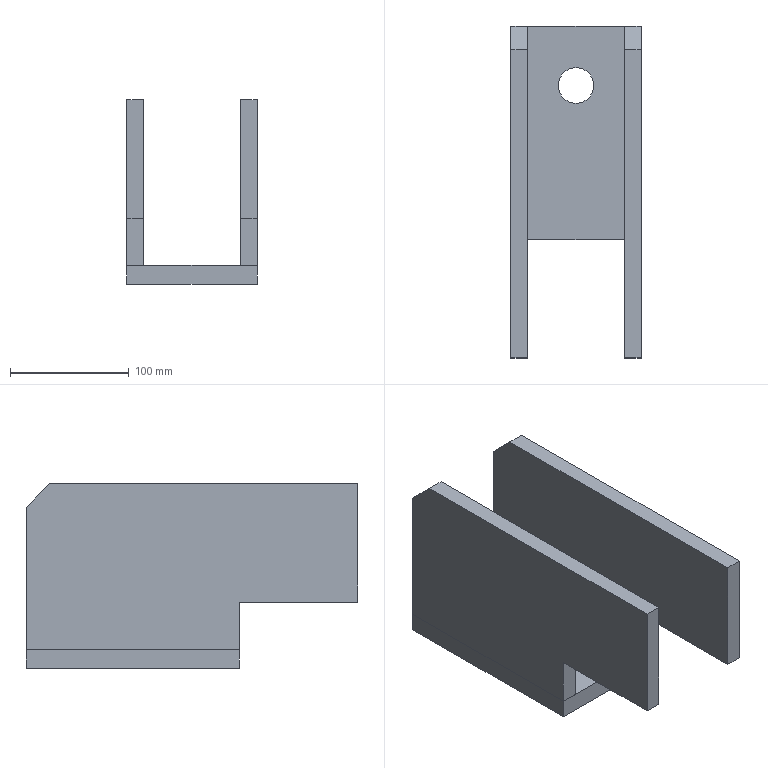Part | SolidWorks | features ICE 3, Chamfer 1, Extrusion 1, MirrorSolid 1, WeldmentFeature 1 | 3 solids | 26 faces | box 110 x 280 x 156 mm | volume 1285490 mm3 | plane 24 | cylinder 2 | commonest cylinder face diameters 30 x2
STEP:
#1=CARTESIAN_POINT('',(-55.,50.,136.));
#2=VERTEX_POINT('',#1);
#3=CARTESIAN_POINT('',(-55.,50.,16.));
#4=VERTEX_POINT('',#3);
#5=CARTESIAN_POINT('',(-55.,50.,16.));
#6=DIRECTION('',(0.,0.,-1.));
#7=VECTOR('',#6,1000.);
#8=LINE('',#5,#7);
#9=EDGE_CURVE('',#2,#4,#8,.T.);
#10=ORIENTED_EDGE('',*,*,#9,.F.);
#11=CARTESIAN_POINT('',(-41.,50.,136.));
#12=VERTEX_POINT('',#11);
#13=CARTESIAN_POINT('',(-41.,50.,136.));
#14=DIRECTION('',(1.,0.,0.));
#15=VECTOR('',#14,1000.);
#16=LINE('',#13,#15);
#17=EDGE_CURVE('',#2,#12,#16,.T.);
#18=ORIENTED_EDGE('',*,*,#17,.T.);
#19=CARTESIAN_POINT('',(-41.,50.,16.));
#20=VERTEX_POINT('',#19);
#21=CARTESIAN_POINT('',(-41.,50.,16.));
#22=DIRECTION('',(0.,0.,-1.));
#23=VECTOR('',#22,1000.);
#24=LINE('',#21,#23);
#25=EDGE_CURVE('',#12,#20,#24,.T.);
#26=ORIENTED_EDGE('',*,*,#25,.T.);
#27=CARTESIAN_POINT('',(-41.,50.,16.));
#28=DIRECTION('',(-1.,0.,0.));
#29=VECTOR('',#28,1000.);
#30=LINE('',#27,#29);
#31=EDGE_CURVE('',#20,#4,#30,.T.);
#32=ORIENTED_EDGE('',*,*,#31,.T.);
#33=EDGE_LOOP('',(#10,#18,#26,#32));
#34=FACE_OUTER_BOUND('',#33,.T.);
#35=CARTESIAN_POINT('',(-41.,50.,16.));
#36=DIRECTION('',(0.,1.,0.));
#37=DIRECTION('',(0.,0.,1.));
#38=AXIS2_PLACEMENT_3D('',#35,#36,#37);
#39=PLANE('',#38);
#40=ADVANCED_FACE('',(#34),#39,.T.);
#41=CARTESIAN_POINT('',(-41.,-230.,156.));
#42=VERTEX_POINT('',#41);
#43=CARTESIAN_POINT('',(-41.,30.,156.));
#44=VERTEX_POINT('',#43);
#45=CARTESIAN_POINT('',(-41.,50.,156.));
#46=DIRECTION('',(0.,1.,0.));
#47=VECTOR('',#46,1000.);
#48=LINE('',#45,#47);
#49=EDGE_CURVE('',#42,#44,#48,.T.);
#50=ORIENTED_EDGE('',*,*,#49,.T.);
#51=CARTESIAN_POINT('',(-55.,30.,156.));
#52=VERTEX_POINT('',#51);
#53=CARTESIAN_POINT('',(-41.,30.,156.));
#54=DIRECTION('',(-1.,0.,0.));
#55=VECTOR('',#54,1000.);
#56=LINE('',#53,#55);
#57=EDGE_CURVE('',#44,#52,#56,.T.);
#58=ORIENTED_EDGE('',*,*,#57,.T.);
#59=CARTESIAN_POINT('',(-55.,-230.,156.));
#60=VERTEX_POINT('',#59);
#61=CARTESIAN_POINT('',(-55.,50.,156.));
#62=DIRECTION('',(0.,1.,0.));
#63=VECTOR('',#62,1000.);
#64=LINE('',#61,#63);
#65=EDGE_CURVE('',#60,#52,#64,.T.);
#66=ORIENTED_EDGE('',*,*,#65,.F.);
#67=CARTESIAN_POINT('',(-41.,-230.,156.));
#68=DIRECTION('',(-1.,0.,0.));
#69=VECTOR('',#68,1000.);
#70=LINE('',#67,#69);
#71=EDGE_CURVE('',#42,#60,#70,.T.);
#72=ORIENTED_EDGE('',*,*,#71,.F.);
#73=EDGE_LOOP('',(#50,#58,#66,#72));
#74=FACE_OUTER_BOUND('',#73,.T.);
#75=CARTESIAN_POINT('',(-41.,50.,156.));
#76=DIRECTION('',(0.,0.,1.));
#77=DIRECTION('',(0.,-1.,0.));
#78=AXIS2_PLACEMENT_3D('',#75,#76,#77);
#79=PLANE('',#78);
#80=ADVANCED_FACE('',(#74),#79,.T.);
#81=CARTESIAN_POINT('',(-55.,-230.,56.));
#82=VERTEX_POINT('',#81);
#83=CARTESIAN_POINT('',(-55.,-230.,156.));
#84=DIRECTION('',(0.,0.,1.));
#85=VECTOR('',#84,1000.);
#86=LINE('',#83,#85);
#87=EDGE_CURVE('',#82,#60,#86,.T.);
#88=ORIENTED_EDGE('',*,*,#87,.F.);
#89=CARTESIAN_POINT('',(-41.,-230.,56.));
#90=VERTEX_POINT('',#89);
#91=CARTESIAN_POINT('',(-41.,-230.,56.));
#92=DIRECTION('',(-1.,0.,0.));
#93=VECTOR('',#92,1000.);
#94=LINE('',#91,#93);
#95=EDGE_CURVE('',#90,#82,#94,.T.);
#96=ORIENTED_EDGE('',*,*,#95,.F.);
#97=CARTESIAN_POINT('',(-41.,-230.,156.));
#98=DIRECTION('',(0.,0.,1.));
#99=VECTOR('',#98,1000.);
#100=LINE('',#97,#99);
#101=EDGE_CURVE('',#90,#42,#100,.T.);
#102=ORIENTED_EDGE('',*,*,#101,.T.);
#103=ORIENTED_EDGE('',*,*,#71,.T.);
#104=EDGE_LOOP('',(#88,#96,#102,#103));
#105=FACE_OUTER_BOUND('',#104,.T.);
#106=CARTESIAN_POINT('',(-41.,-230.,156.));
#107=DIRECTION('',(0.,-1.,0.));
#108=DIRECTION('',(0.,0.,-1.));
#109=AXIS2_PLACEMENT_3D('',#106,#107,#108);
#110=PLANE('',#109);
#111=ADVANCED_FACE('',(#105),#110,.T.);
#112=CARTESIAN_POINT('',(-55.,-130.,56.));
#113=VERTEX_POINT('',#112);
#114=CARTESIAN_POINT('',(-55.,-230.,56.));
#115=DIRECTION('',(0.,-1.,0.));
#116=VECTOR('',#115,1000.);
#117=LINE('',#114,#116);
#118=EDGE_CURVE('',#113,#82,#117,.T.);
#119=ORIENTED_EDGE('',*,*,#118,.F.);
#120=CARTESIAN_POINT('',(-41.,-130.,56.));
#121=VERTEX_POINT('',#120);
#122=CARTESIAN_POINT('',(-41.,-130.,56.));
#123=DIRECTION('',(-1.,0.,0.));
#124=VECTOR('',#123,1000.);
#125=LINE('',#122,#124);
#126=EDGE_CURVE('',#121,#113,#125,.T.);
#127=ORIENTED_EDGE('',*,*,#126,.F.);
#128=CARTESIAN_POINT('',(-41.,-230.,56.));
#129=DIRECTION('',(0.,-1.,0.));
#130=VECTOR('',#129,1000.);
#131=LINE('',#128,#130);
#132=EDGE_CURVE('',#121,#90,#131,.T.);
#133=ORIENTED_EDGE('',*,*,#132,.T.);
#134=ORIENTED_EDGE('',*,*,#95,.T.);
#135=EDGE_LOOP('',(#119,#127,#133,#134));
#136=FACE_OUTER_BOUND('',#135,.T.);
#137=CARTESIAN_POINT('',(-41.,-230.,56.));
#138=DIRECTION('',(0.,0.,-1.));
#139=DIRECTION('',(-1.,0.,0.));
#140=AXIS2_PLACEMENT_3D('',#137,#138,#139);
#141=PLANE('',#140);
#142=ADVANCED_FACE('',(#136),#141,.T.);
#143=CARTESIAN_POINT('',(-55.,-130.,16.));
#144=VERTEX_POINT('',#143);
#145=CARTESIAN_POINT('',(-55.,-130.,56.));
#146=DIRECTION('',(0.,0.,1.));
#147=VECTOR('',#146,1000.);
#148=LINE('',#145,#147);
#149=EDGE_CURVE('',#144,#113,#148,.T.);
#150=ORIENTED_EDGE('',*,*,#149,.F.);
#151=CARTESIAN_POINT('',(-41.,-130.,16.));
#152=VERTEX_POINT('',#151);
#153=CARTESIAN_POINT('',(-41.,-130.,16.));
#154=DIRECTION('',(-1.,0.,0.));
#155=VECTOR('',#154,1000.);
#156=LINE('',#153,#155);
#157=EDGE_CURVE('',#152,#144,#156,.T.);
#158=ORIENTED_EDGE('',*,*,#157,.F.);
#159=CARTESIAN_POINT('',(-41.,-130.,56.));
#160=DIRECTION('',(0.,0.,1.));
#161=VECTOR('',#160,1000.);
#162=LINE('',#159,#161);
#163=EDGE_CURVE('',#152,#121,#162,.T.);
#164=ORIENTED_EDGE('',*,*,#163,.T.);
#165=ORIENTED_EDGE('',*,*,#126,.T.);
#166=EDGE_LOOP('',(#150,#158,#164,#165));
#167=FACE_OUTER_BOUND('',#166,.T.);
#168=CARTESIAN_POINT('',(-41.,-130.,56.));
#169=DIRECTION('',(0.,-1.,0.));
#170=DIRECTION('',(0.,0.,-1.));
#171=AXIS2_PLACEMENT_3D('',#168,#169,#170);
#172=PLANE('',#171);
#173=ADVANCED_FACE('',(#167),#172,.T.);
#174=CARTESIAN_POINT('',(-55.,50.,16.));
#175=DIRECTION('',(0.,-1.,0.));
#176=VECTOR('',#175,1000.);
#177=LINE('',#174,#176);
#178=EDGE_CURVE('',#4,#144,#177,.T.);
#179=ORIENTED_EDGE('',*,*,#178,.F.);
#180=ORIENTED_EDGE('',*,*,#31,.F.);
#181=CARTESIAN_POINT('',(-41.,50.,16.));
#182=DIRECTION('',(0.,-1.,0.));
#183=VECTOR('',#182,1000.);
#184=LINE('',#181,#183);
#185=EDGE_CURVE('',#20,#152,#184,.T.);
#186=ORIENTED_EDGE('',*,*,#185,.T.);
#187=ORIENTED_EDGE('',*,*,#157,.T.);
#188=EDGE_LOOP('',(#179,#180,#186,#187));
#189=FACE_OUTER_BOUND('',#188,.T.);
#190=CARTESIAN_POINT('',(-41.,50.,16.));
#191=DIRECTION('',(0.,0.,-1.));
#192=DIRECTION('',(-1.,0.,0.));
#193=AXIS2_PLACEMENT_3D('',#190,#191,#192);
#194=PLANE('',#193);
#195=ADVANCED_FACE('',(#189),#194,.T.);
#196=ORIENTED_EDGE('',*,*,#25,.F.);
#197=CARTESIAN_POINT('',(-41.,93.,93.));
#198=DIRECTION('',(0.,-0.7071,0.7071));
#199=VECTOR('',#198,1000.);
#200=LINE('',#197,#199);
#201=EDGE_CURVE('',#12,#44,#200,.T.);
#202=ORIENTED_EDGE('',*,*,#201,.T.);
#203=ORIENTED_EDGE('',*,*,#49,.F.);
#204=ORIENTED_EDGE('',*,*,#101,.F.);
#205=ORIENTED_EDGE('',*,*,#132,.F.);
#206=ORIENTED_EDGE('',*,*,#163,.F.);
#207=ORIENTED_EDGE('',*,*,#185,.F.);
#208=EDGE_LOOP('',(#196,#202,#203,#204,#205,#206,#207));
#209=FACE_OUTER_BOUND('',#208,.T.);
#210=CARTESIAN_POINT('',(-41.,0.,0.));
#211=DIRECTION('',(1.,0.,0.));
#212=DIRECTION('',(0.,0.,-1.));
#213=AXIS2_PLACEMENT_3D('',#210,#211,#212);
#214=PLANE('',#213);
#215=ADVANCED_FACE('',(#209),#214,.T.);
#216=ORIENTED_EDGE('',*,*,#65,.T.);
#217=CARTESIAN_POINT('',(-55.,30.,156.));
#218=DIRECTION('',(0.,0.7071,-0.7071));
#219=VECTOR('',#218,1000.);
#220=LINE('',#217,#219);
#221=EDGE_CURVE('',#52,#2,#220,.T.);
#222=ORIENTED_EDGE('',*,*,#221,.T.);
#223=ORIENTED_EDGE('',*,*,#9,.T.);
#224=ORIENTED_EDGE('',*,*,#178,.T.);
#225=ORIENTED_EDGE('',*,*,#149,.T.);
#226=ORIENTED_EDGE('',*,*,#118,.T.);
#227=ORIENTED_EDGE('',*,*,#87,.T.);
#228=EDGE_LOOP('',(#216,#222,#223,#224,#225,#226,#227));
#229=FACE_OUTER_BOUND('',#228,.T.);
#230=CARTESIAN_POINT('',(-55.,0.,0.));
#231=DIRECTION('',(1.,0.,0.));
#232=DIRECTION('',(0.,0.,-1.));
#233=AXIS2_PLACEMENT_3D('',#230,#231,#232);
#234=PLANE('',#233);
#235=ADVANCED_FACE('',(#229),#234,.F.);
#236=ORIENTED_EDGE('',*,*,#201,.F.);
#237=ORIENTED_EDGE('',*,*,#17,.F.);
#238=ORIENTED_EDGE('',*,*,#221,.F.);
#239=ORIENTED_EDGE('',*,*,#57,.F.);
#240=EDGE_LOOP('',(#236,#237,#238,#239));
#241=FACE_OUTER_BOUND('',#240,.T.);
#242=CARTESIAN_POINT('',(-41.,30.,156.));
#243=DIRECTION('',(0.,-0.7071,-0.7071));
#244=DIRECTION('',(-1.,0.,0.));
#245=AXIS2_PLACEMENT_3D('',#242,#243,#244);
#246=PLANE('',#245);
#247=ADVANCED_FACE('',(#241),#246,.F.);
#248=CLOSED_SHELL('',(#40,#80,#111,#142,#173,#195,#215,#235,#247));
#249=MANIFOLD_SOLID_BREP('',#248);
#250=CARTESIAN_POINT('',(55.,50.,136.));
#251=VERTEX_POINT('',#250);
#252=CARTESIAN_POINT('',(55.,50.,16.));
#253=VERTEX_POINT('',#252);
#254=CARTESIAN_POINT('',(55.,50.,16.));
#255=DIRECTION('',(0.,0.,-1.));
#256=VECTOR('',#255,1000.);
#257=LINE('',#254,#256);
#258=EDGE_CURVE('',#251,#253,#257,.T.);
#259=ORIENTED_EDGE('',*,*,#258,.T.);
#260=CARTESIAN_POINT('',(41.,50.,16.));
#261=VERTEX_POINT('',#260);
#262=CARTESIAN_POINT('',(41.,50.,16.));
#263=DIRECTION('',(1.,0.,0.));
#264=VECTOR('',#263,1000.);
#265=LINE('',#262,#264);
#266=EDGE_CURVE('',#261,#253,#265,.T.);
#267=ORIENTED_EDGE('',*,*,#266,.F.);
#268=CARTESIAN_POINT('',(41.,50.,136.));
#269=VERTEX_POINT('',#268);
#270=CARTESIAN_POINT('',(41.,50.,16.));
#271=DIRECTION('',(0.,0.,-1.));
#272=VECTOR('',#271,1000.);
#273=LINE('',#270,#272);
#274=EDGE_CURVE('',#269,#261,#273,.T.);
#275=ORIENTED_EDGE('',*,*,#274,.F.);
#276=CARTESIAN_POINT('',(41.,50.,136.));
#277=DIRECTION('',(-1.,0.,0.));
#278=VECTOR('',#277,1000.);
#279=LINE('',#276,#278);
#280=EDGE_CURVE('',#251,#269,#279,.T.);
#281=ORIENTED_EDGE('',*,*,#280,.F.);
#282=EDGE_LOOP('',(#259,#267,#275,#281));
#283=FACE_OUTER_BOUND('',#282,.T.);
#284=CARTESIAN_POINT('',(41.,50.,16.));
#285=DIRECTION('',(0.,1.,0.));
#286=DIRECTION('',(0.,0.,1.));
#287=AXIS2_PLACEMENT_3D('',#284,#285,#286);
#288=PLANE('',#287);
#289=ADVANCED_FACE('',(#283),#288,.T.);
#290=CARTESIAN_POINT('',(41.,-230.,156.));
#291=VERTEX_POINT('',#290);
#292=CARTESIAN_POINT('',(41.,30.,156.));
#293=VERTEX_POINT('',#292);
#294=CARTESIAN_POINT('',(41.,50.,156.));
#295=DIRECTION('',(0.,1.,0.));
#296=VECTOR('',#295,1000.);
#297=LINE('',#294,#296);
#298=EDGE_CURVE('',#291,#293,#297,.T.);
#299=ORIENTED_EDGE('',*,*,#298,.F.);
#300=CARTESIAN_POINT('',(55.,-230.,156.));
#301=VERTEX_POINT('',#300);
#302=CARTESIAN_POINT('',(41.,-230.,156.));
#303=DIRECTION('',(1.,0.,0.));
#304=VECTOR('',#303,1000.);
#305=LINE('',#302,#304);
#306=EDGE_CURVE('',#291,#301,#305,.T.);
#307=ORIENTED_EDGE('',*,*,#306,.T.);
#308=CARTESIAN_POINT('',(55.,30.,156.));
#309=VERTEX_POINT('',#308);
#310=CARTESIAN_POINT('',(55.,50.,156.));
#311=DIRECTION('',(0.,1.,0.));
#312=VECTOR('',#311,1000.);
#313=LINE('',#310,#312);
#314=EDGE_CURVE('',#301,#309,#313,.T.);
#315=ORIENTED_EDGE('',*,*,#314,.T.);
#316=CARTESIAN_POINT('',(41.,30.,156.));
#317=DIRECTION('',(1.,0.,0.));
#318=VECTOR('',#317,1000.);
#319=LINE('',#316,#318);
#320=EDGE_CURVE('',#293,#309,#319,.T.);
#321=ORIENTED_EDGE('',*,*,#320,.F.);
#322=EDGE_LOOP('',(#299,#307,#315,#321));
#323=FACE_OUTER_BOUND('',#322,.T.);
#324=CARTESIAN_POINT('',(41.,50.,156.));
#325=DIRECTION('',(0.,0.,1.));
#326=DIRECTION('',(0.,-1.,0.));
#327=AXIS2_PLACEMENT_3D('',#324,#325,#326);
#328=PLANE('',#327);
#329=ADVANCED_FACE('',(#323),#328,.T.);
#330=CARTESIAN_POINT('',(55.,-230.,56.));
#331=VERTEX_POINT('',#330);
#332=CARTESIAN_POINT('',(55.,-230.,156.));
#333=DIRECTION('',(0.,0.,1.));
#334=VECTOR('',#333,1000.);
#335=LINE('',#332,#334);
#336=EDGE_CURVE('',#331,#301,#335,.T.);
#337=ORIENTED_EDGE('',*,*,#336,.T.);
#338=ORIENTED_EDGE('',*,*,#306,.F.);
#339=CARTESIAN_POINT('',(41.,-230.,56.));
#340=VERTEX_POINT('',#339);
#341=CARTESIAN_POINT('',(41.,-230.,156.));
#342=DIRECTION('',(0.,0.,1.));
#343=VECTOR('',#342,1000.);
#344=LINE('',#341,#343);
#345=EDGE_CURVE('',#340,#291,#344,.T.);
#346=ORIENTED_EDGE('',*,*,#345,.F.);
#347=CARTESIAN_POINT('',(41.,-230.,56.));
#348=DIRECTION('',(1.,0.,0.));
#349=VECTOR('',#348,1000.);
#350=LINE('',#347,#349);
#351=EDGE_CURVE('',#340,#331,#350,.T.);
#352=ORIENTED_EDGE('',*,*,#351,.T.);
#353=EDGE_LOOP('',(#337,#338,#346,#352));
#354=FACE_OUTER_BOUND('',#353,.T.);
#355=CARTESIAN_POINT('',(41.,-230.,156.));
#356=DIRECTION('',(0.,-1.,0.));
#357=DIRECTION('',(0.,0.,-1.));
#358=AXIS2_PLACEMENT_3D('',#355,#356,#357);
#359=PLANE('',#358);
#360=ADVANCED_FACE('',(#354),#359,.T.);
#361=CARTESIAN_POINT('',(55.,-130.,56.));
#362=VERTEX_POINT('',#361);
#363=CARTESIAN_POINT('',(55.,-230.,56.));
#364=DIRECTION('',(0.,-1.,0.));
#365=VECTOR('',#364,1000.);
#366=LINE('',#363,#365);
#367=EDGE_CURVE('',#362,#331,#366,.T.);
#368=ORIENTED_EDGE('',*,*,#367,.T.);
#369=ORIENTED_EDGE('',*,*,#351,.F.);
#370=CARTESIAN_POINT('',(41.,-130.,56.));
#371=VERTEX_POINT('',#370);
#372=CARTESIAN_POINT('',(41.,-230.,56.));
#373=DIRECTION('',(0.,-1.,0.));
#374=VECTOR('',#373,1000.);
#375=LINE('',#372,#374);
#376=EDGE_CURVE('',#371,#340,#375,.T.);
#377=ORIENTED_EDGE('',*,*,#376,.F.);
#378=CARTESIAN_POINT('',(41.,-130.,56.));
#379=DIRECTION('',(1.,0.,0.));
#380=VECTOR('',#379,1000.);
#381=LINE('',#378,#380);
#382=EDGE_CURVE('',#371,#362,#381,.T.);
#383=ORIENTED_EDGE('',*,*,#382,.T.);
#384=EDGE_LOOP('',(#368,#369,#377,#383));
#385=FACE_OUTER_BOUND('',#384,.T.);
#386=CARTESIAN_POINT('',(41.,-230.,56.));
#387=DIRECTION('',(0.,0.,-1.));
#388=DIRECTION('',(1.,0.,0.));
#389=AXIS2_PLACEMENT_3D('',#386,#387,#388);
#390=PLANE('',#389);
#391=ADVANCED_FACE('',(#385),#390,.T.);
#392=CARTESIAN_POINT('',(55.,-130.,16.));
#393=VERTEX_POINT('',#392);
#394=CARTESIAN_POINT('',(55.,-130.,56.));
#395=DIRECTION('',(0.,0.,1.));
#396=VECTOR('',#395,1000.);
#397=LINE('',#394,#396);
#398=EDGE_CURVE('',#393,#362,#397,.T.);
#399=ORIENTED_EDGE('',*,*,#398,.T.);
#400=ORIENTED_EDGE('',*,*,#382,.F.);
#401=CARTESIAN_POINT('',(41.,-130.,16.));
#402=VERTEX_POINT('',#401);
#403=CARTESIAN_POINT('',(41.,-130.,56.));
#404=DIRECTION('',(0.,0.,1.));
#405=VECTOR('',#404,1000.);
#406=LINE('',#403,#405);
#407=EDGE_CURVE('',#402,#371,#406,.T.);
#408=ORIENTED_EDGE('',*,*,#407,.F.);
#409=CARTESIAN_POINT('',(41.,-130.,16.));
#410=DIRECTION('',(1.,0.,0.));
#411=VECTOR('',#410,1000.);
#412=LINE('',#409,#411);
#413=EDGE_CURVE('',#402,#393,#412,.T.);
#414=ORIENTED_EDGE('',*,*,#413,.T.);
#415=EDGE_LOOP('',(#399,#400,#408,#414));
#416=FACE_OUTER_BOUND('',#415,.T.);
#417=CARTESIAN_POINT('',(41.,-130.,56.));
#418=DIRECTION('',(0.,-1.,0.));
#419=DIRECTION('',(0.,0.,-1.));
#420=AXIS2_PLACEMENT_3D('',#417,#418,#419);
#421=PLANE('',#420);
#422=ADVANCED_FACE('',(#416),#421,.T.);
#423=CARTESIAN_POINT('',(55.,50.,16.));
#424=DIRECTION('',(0.,-1.,0.));
#425=VECTOR('',#424,1000.);
#426=LINE('',#423,#425);
#427=EDGE_CURVE('',#253,#393,#426,.T.);
#428=ORIENTED_EDGE('',*,*,#427,.T.);
#429=ORIENTED_EDGE('',*,*,#413,.F.);
#430=CARTESIAN_POINT('',(41.,50.,16.));
#431=DIRECTION('',(0.,-1.,0.));
#432=VECTOR('',#431,1000.);
#433=LINE('',#430,#432);
#434=EDGE_CURVE('',#261,#402,#433,.T.);
#435=ORIENTED_EDGE('',*,*,#434,.F.);
#436=ORIENTED_EDGE('',*,*,#266,.T.);
#437=EDGE_LOOP('',(#428,#429,#435,#436));
#438=FACE_OUTER_BOUND('',#437,.T.);
#439=CARTESIAN_POINT('',(41.,50.,16.));
#440=DIRECTION('',(0.,0.,-1.));
#441=DIRECTION('',(1.,0.,0.));
#442=AXIS2_PLACEMENT_3D('',#439,#440,#441);
#443=PLANE('',#442);
#444=ADVANCED_FACE('',(#438),#443,.T.);
#445=ORIENTED_EDGE('',*,*,#274,.T.);
#446=ORIENTED_EDGE('',*,*,#434,.T.);
#447=ORIENTED_EDGE('',*,*,#407,.T.);
#448=ORIENTED_EDGE('',*,*,#376,.T.);
#449=ORIENTED_EDGE('',*,*,#345,.T.);
#450=ORIENTED_EDGE('',*,*,#298,.T.);
#451=CARTESIAN_POINT('',(41.,93.,93.));
#452=DIRECTION('',(0.,-0.7071,0.7071));
#453=VECTOR('',#452,1000.);
#454=LINE('',#451,#453);
#455=EDGE_CURVE('',#269,#293,#454,.T.);
#456=ORIENTED_EDGE('',*,*,#455,.F.);
#457=EDGE_LOOP('',(#445,#446,#447,#448,#449,#450,#456));
#458=FACE_OUTER_BOUND('',#457,.T.);
#459=CARTESIAN_POINT('',(41.,0.,0.));
#460=DIRECTION('',(-1.,0.,0.));
#461=DIRECTION('',(0.,0.,-1.));
#462=AXIS2_PLACEMENT_3D('',#459,#460,#461);
#463=PLANE('',#462);
#464=ADVANCED_FACE('',(#458),#463,.T.);
#465=ORIENTED_EDGE('',*,*,#314,.F.);
#466=ORIENTED_EDGE('',*,*,#336,.F.);
#467=ORIENTED_EDGE('',*,*,#367,.F.);
#468=ORIENTED_EDGE('',*,*,#398,.F.);
#469=ORIENTED_EDGE('',*,*,#427,.F.);
#470=ORIENTED_EDGE('',*,*,#258,.F.);
#471=CARTESIAN_POINT('',(55.,30.,156.));
#472=DIRECTION('',(0.,0.7071,-0.7071));
#473=VECTOR('',#472,1000.);
#474=LINE('',#471,#473);
#475=EDGE_CURVE('',#309,#251,#474,.T.);
#476=ORIENTED_EDGE('',*,*,#475,.F.);
#477=EDGE_LOOP('',(#465,#466,#467,#468,#469,#470,#476));
#478=FACE_OUTER_BOUND('',#477,.T.);
#479=CARTESIAN_POINT('',(55.,0.,0.));
#480=DIRECTION('',(-1.,0.,0.));
#481=DIRECTION('',(0.,0.,-1.));
#482=AXIS2_PLACEMENT_3D('',#479,#480,#481);
#483=PLANE('',#482);
#484=ADVANCED_FACE('',(#478),#483,.F.);
#485=ORIENTED_EDGE('',*,*,#455,.T.);
#486=ORIENTED_EDGE('',*,*,#320,.T.);
#487=ORIENTED_EDGE('',*,*,#475,.T.);
#488=ORIENTED_EDGE('',*,*,#280,.T.);
#489=EDGE_LOOP('',(#485,#486,#487,#488));
#490=FACE_OUTER_BOUND('',#489,.T.);
#491=CARTESIAN_POINT('',(41.,30.,156.));
#492=DIRECTION('',(0.,-0.7071,-0.7071));
#493=DIRECTION('',(1.,0.,0.));
#494=AXIS2_PLACEMENT_3D('',#491,#492,#493);
#495=PLANE('',#494);
#496=ADVANCED_FACE('',(#490),#495,.F.);
#497=CLOSED_SHELL('',(#289,#329,#360,#391,#422,#444,#464,#484,#496));
#498=MANIFOLD_SOLID_BREP('',#497);
#499=CARTESIAN_POINT('',(-15.,0.,16.));
#500=VERTEX_POINT('',#499);
#501=CARTESIAN_POINT('',(15.,0.,16.));
#502=VERTEX_POINT('',#501);
#503=CARTESIAN_POINT('',(0.,0.,16.));
#504=DIRECTION('',(0.,0.,1.));
#505=DIRECTION('',(-1.,0.,0.));
#506=AXIS2_PLACEMENT_3D('',#503,#504,#505);
#507=CIRCLE('',#506,15.);
#508=EDGE_CURVE('',#500,#502,#507,.T.);
#509=ORIENTED_EDGE('',*,*,#508,.T.);
#510=CARTESIAN_POINT('',(15.,0.,0.));
#511=VERTEX_POINT('',#510);
#512=CARTESIAN_POINT('',(15.,0.,156.001));
#513=DIRECTION('',(0.,0.,-1.));
#514=VECTOR('',#513,1000.);
#515=LINE('',#512,#514);
#516=EDGE_CURVE('',#502,#511,#515,.T.);
#517=ORIENTED_EDGE('',*,*,#516,.T.);
#518=CARTESIAN_POINT('',(-15.,0.,0.));
#519=VERTEX_POINT('',#518);
#520=CARTESIAN_POINT('',(0.,0.,0.));
#521=DIRECTION('',(0.,0.,-1.));
#522=DIRECTION('',(-1.,0.,0.));
#523=AXIS2_PLACEMENT_3D('',#520,#521,#522);
#524=CIRCLE('',#523,15.);
#525=EDGE_CURVE('',#511,#519,#524,.T.);
#526=ORIENTED_EDGE('',*,*,#525,.T.);
#527=CARTESIAN_POINT('',(-15.,0.,156.001));
#528=DIRECTION('',(0.,0.,-1.));
#529=VECTOR('',#528,1000.);
#530=LINE('',#527,#529);
#531=EDGE_CURVE('',#500,#519,#530,.T.);
#532=ORIENTED_EDGE('',*,*,#531,.F.);
#533=EDGE_LOOP('',(#509,#517,#526,#532));
#534=FACE_OUTER_BOUND('',#533,.T.);
#535=CARTESIAN_POINT('',(0.,0.,156.001));
#536=DIRECTION('',(0.,0.,-1.));
#537=DIRECTION('',(-1.,0.,0.));
#538=AXIS2_PLACEMENT_3D('',#535,#536,#537);
#539=CYLINDRICAL_SURFACE('',#538,15.);
#540=ADVANCED_FACE('',(#534),#539,.F.);
#541=CARTESIAN_POINT('',(55.,-130.,0.));
#542=VERTEX_POINT('',#541);
#543=CARTESIAN_POINT('',(55.,50.,0.));
#544=VERTEX_POINT('',#543);
#545=CARTESIAN_POINT('',(55.,-50.,0.));
#546=DIRECTION('',(0.,1.,0.));
#547=VECTOR('',#546,1000.);
#548=LINE('',#545,#547);
#549=EDGE_CURVE('',#542,#544,#548,.T.);
#550=ORIENTED_EDGE('',*,*,#549,.T.);
#551=CARTESIAN_POINT('',(55.,50.,16.));
#552=VERTEX_POINT('',#551);
#553=CARTESIAN_POINT('',(55.,50.,16.));
#554=DIRECTION('',(0.,0.,-1.));
#555=VECTOR('',#554,1000.);
#556=LINE('',#553,#555);
#557=EDGE_CURVE('',#552,#544,#556,.T.);
#558=ORIENTED_EDGE('',*,*,#557,.F.);
#559=CARTESIAN_POINT('',(55.,-130.,16.));
#560=VERTEX_POINT('',#559);
#561=CARTESIAN_POINT('',(55.,-50.,16.));
#562=DIRECTION('',(0.,1.,0.));
#563=VECTOR('',#562,1000.);
#564=LINE('',#561,#563);
#565=EDGE_CURVE('',#560,#552,#564,.T.);
#566=ORIENTED_EDGE('',*,*,#565,.F.);
#567=CARTESIAN_POINT('',(55.,-130.,16.));
#568=DIRECTION('',(0.,0.,1.));
#569=VECTOR('',#568,1000.);
#570=LINE('',#567,#569);
#571=EDGE_CURVE('',#542,#560,#570,.T.);
#572=ORIENTED_EDGE('',*,*,#571,.F.);
#573=EDGE_LOOP('',(#550,#558,#566,#572));
#574=FACE_OUTER_BOUND('',#573,.T.);
#575=CARTESIAN_POINT('',(55.,-50.,16.));
#576=DIRECTION('',(-1.,0.,0.));
#577=DIRECTION('',(0.,0.,1.));
#578=AXIS2_PLACEMENT_3D('',#575,#576,#577);
#579=PLANE('',#578);
#580=ADVANCED_FACE('',(#574),#579,.F.);
#581=CARTESIAN_POINT('',(-55.,50.,0.));
#582=VERTEX_POINT('',#581);
#583=CARTESIAN_POINT('',(-55.,50.,0.));
#584=DIRECTION('',(-1.,0.,0.));
#585=VECTOR('',#584,1000.);
#586=LINE('',#583,#585);
#587=EDGE_CURVE('',#544,#582,#586,.T.);
#588=ORIENTED_EDGE('',*,*,#587,.T.);
#589=CARTESIAN_POINT('',(-55.,50.,16.));
#590=VERTEX_POINT('',#589);
#591=CARTESIAN_POINT('',(-55.,50.,16.));
#592=DIRECTION('',(0.,0.,-1.));
#593=VECTOR('',#592,1000.);
#594=LINE('',#591,#593);
#595=EDGE_CURVE('',#590,#582,#594,.T.);
#596=ORIENTED_EDGE('',*,*,#595,.F.);
#597=CARTESIAN_POINT('',(-55.,50.,16.));
#598=DIRECTION('',(-1.,0.,0.));
#599=VECTOR('',#598,1000.);
#600=LINE('',#597,#599);
#601=EDGE_CURVE('',#552,#590,#600,.T.);
#602=ORIENTED_EDGE('',*,*,#601,.F.);
#603=ORIENTED_EDGE('',*,*,#557,.T.);
#604=EDGE_LOOP('',(#588,#596,#602,#603));
#605=FACE_OUTER_BOUND('',#604,.T.);
#606=CARTESIAN_POINT('',(-55.,50.,16.));
#607=DIRECTION('',(0.,-1.,0.));
#608=DIRECTION('',(0.,0.,-1.));
#609=AXIS2_PLACEMENT_3D('',#606,#607,#608);
#610=PLANE('',#609);
#611=ADVANCED_FACE('',(#605),#610,.F.);
#612=CARTESIAN_POINT('',(-55.,-130.,0.));
#613=VERTEX_POINT('',#612);
#614=CARTESIAN_POINT('',(-55.,-50.,0.));
#615=DIRECTION('',(0.,-1.,0.));
#616=VECTOR('',#615,1000.);
#617=LINE('',#614,#616);
#618=EDGE_CURVE('',#582,#613,#617,.T.);
#619=ORIENTED_EDGE('',*,*,#618,.T.);
#620=CARTESIAN_POINT('',(-55.,-130.,16.));
#621=VERTEX_POINT('',#620);
#622=CARTESIAN_POINT('',(-55.,-130.,16.));
#623=DIRECTION('',(0.,0.,-1.));
#624=VECTOR('',#623,1000.);
#625=LINE('',#622,#624);
#626=EDGE_CURVE('',#621,#613,#625,.T.);
#627=ORIENTED_EDGE('',*,*,#626,.F.);
#628=CARTESIAN_POINT('',(-55.,-50.,16.));
#629=DIRECTION('',(0.,-1.,0.));
#630=VECTOR('',#629,1000.);
#631=LINE('',#628,#630);
#632=EDGE_CURVE('',#590,#621,#631,.T.);
#633=ORIENTED_EDGE('',*,*,#632,.F.);
#634=ORIENTED_EDGE('',*,*,#595,.T.);
#635=EDGE_LOOP('',(#619,#627,#633,#634));
#636=FACE_OUTER_BOUND('',#635,.T.);
#637=CARTESIAN_POINT('',(-55.,-50.,16.));
#638=DIRECTION('',(1.,0.,0.));
#639=DIRECTION('',(0.,0.,-1.));
#640=AXIS2_PLACEMENT_3D('',#637,#638,#639);
#641=PLANE('',#640);
#642=ADVANCED_FACE('',(#636),#641,.F.);
#643=ORIENTED_EDGE('',*,*,#508,.F.);
#644=CARTESIAN_POINT('',(0.,0.,16.));
#645=DIRECTION('',(0.,0.,1.));
#646=DIRECTION('',(-1.,0.,0.));
#647=AXIS2_PLACEMENT_3D('',#644,#645,#646);
#648=CIRCLE('',#647,15.);
#649=EDGE_CURVE('',#502,#500,#648,.T.);
#650=ORIENTED_EDGE('',*,*,#649,.F.);
#651=EDGE_LOOP('',(#643,#650));
#652=FACE_BOUND('',#651,.T.);
#653=ORIENTED_EDGE('',*,*,#565,.T.);
#654=ORIENTED_EDGE('',*,*,#601,.T.);
#655=ORIENTED_EDGE('',*,*,#632,.T.);
#656=CARTESIAN_POINT('',(-55.,-130.,16.));
#657=DIRECTION('',(-1.,0.,0.));
#658=VECTOR('',#657,1000.);
#659=LINE('',#656,#658);
#660=EDGE_CURVE('',#560,#621,#659,.T.);
#661=ORIENTED_EDGE('',*,*,#660,.F.);
#662=EDGE_LOOP('',(#653,#654,#655,#661));
#663=FACE_OUTER_BOUND('',#662,.T.);
#664=CARTESIAN_POINT('',(0.,0.,16.));
#665=DIRECTION('',(0.,0.,-1.));
#666=DIRECTION('',(-1.,0.,0.));
#667=AXIS2_PLACEMENT_3D('',#664,#665,#666);
#668=PLANE('',#667);
#669=ADVANCED_FACE('',(#652,#663),#668,.F.);
#670=CARTESIAN_POINT('',(0.,0.,0.));
#671=DIRECTION('',(0.,0.,-1.));
#672=DIRECTION('',(-1.,0.,0.));
#673=AXIS2_PLACEMENT_3D('',#670,#671,#672);
#674=CIRCLE('',#673,15.);
#675=EDGE_CURVE('',#519,#511,#674,.T.);
#676=ORIENTED_EDGE('',*,*,#675,.F.);
#677=ORIENTED_EDGE('',*,*,#525,.F.);
#678=EDGE_LOOP('',(#676,#677));
#679=FACE_BOUND('',#678,.T.);
#680=ORIENTED_EDGE('',*,*,#549,.F.);
#681=CARTESIAN_POINT('',(-55.,-130.,0.));
#682=DIRECTION('',(1.,0.,0.));
#683=VECTOR('',#682,1000.);
#684=LINE('',#681,#683);
#685=EDGE_CURVE('',#613,#542,#684,.T.);
#686=ORIENTED_EDGE('',*,*,#685,.F.);
#687=ORIENTED_EDGE('',*,*,#618,.F.);
#688=ORIENTED_EDGE('',*,*,#587,.F.);
#689=EDGE_LOOP('',(#680,#686,#687,#688));
#690=FACE_OUTER_BOUND('',#689,.T.);
#691=CARTESIAN_POINT('',(0.,0.,0.));
#692=DIRECTION('',(0.,0.,-1.));
#693=DIRECTION('',(-1.,0.,0.));
#694=AXIS2_PLACEMENT_3D('',#691,#692,#693);
#695=PLANE('',#694);
#696=ADVANCED_FACE('',(#679,#690),#695,.T.);
#697=ORIENTED_EDGE('',*,*,#516,.F.);
#698=ORIENTED_EDGE('',*,*,#649,.T.);
#699=ORIENTED_EDGE('',*,*,#531,.T.);
#700=ORIENTED_EDGE('',*,*,#675,.T.);
#701=EDGE_LOOP('',(#697,#698,#699,#700));
#702=FACE_OUTER_BOUND('',#701,.T.);
#703=CARTESIAN_POINT('',(0.,0.,156.001));
#704=DIRECTION('',(0.,0.,-1.));
#705=DIRECTION('',(-1.,0.,0.));
#706=AXIS2_PLACEMENT_3D('',#703,#704,#705);
#707=CYLINDRICAL_SURFACE('',#706,15.);
#708=ADVANCED_FACE('',(#702),#707,.F.);
#709=ORIENTED_EDGE('',*,*,#626,.T.);
#710=ORIENTED_EDGE('',*,*,#685,.T.);
#711=ORIENTED_EDGE('',*,*,#571,.T.);
#712=ORIENTED_EDGE('',*,*,#660,.T.);
#713=EDGE_LOOP('',(#709,#710,#711,#712));
#714=FACE_OUTER_BOUND('',#713,.T.);
#715=CARTESIAN_POINT('',(0.,-130.,0.));
#716=DIRECTION('',(0.,-1.,0.));
#717=DIRECTION('',(0.,0.,-1.));
#718=AXIS2_PLACEMENT_3D('',#715,#716,#717);
#719=PLANE('',#718);
#720=ADVANCED_FACE('',(#714),#719,.T.);
#721=CLOSED_SHELL('',(#540,#580,#611,#642,#669,#696,#708,#720));
#722=MANIFOLD_SOLID_BREP('',#721);
#723=CARTESIAN_POINT('',(0.,0.,0.));
#724=DIRECTION('',(0.,0.,1.));
#725=DIRECTION('',(1.,0.,0.));
#726=AXIS2_PLACEMENT_3D('',#723,#724,#725);
#727=(LENGTH_UNIT()NAMED_UNIT(*)SI_UNIT(.MILLI.,.METRE.));
#728=UNCERTAINTY_MEASURE_WITH_UNIT(LENGTH_MEASURE(0.00001),#727,'','');
#729=(NAMED_UNIT(*)PLANE_ANGLE_UNIT()SI_UNIT($,.RADIAN.));
#730=(NAMED_UNIT(*)SI_UNIT($,.STERADIAN.)SOLID_ANGLE_UNIT());
#731=(GEOMETRIC_REPRESENTATION_CONTEXT(3)GLOBAL_UNCERTAINTY_ASSIGNED_CONTEXT((#728))GLOBAL_UNIT_ASSIGNED_CONTEXT((#727,#729,#730))REPRESENTATION_CONTEXT('',''));
#732=ADVANCED_BREP_SHAPE_REPRESENTATION('',(#249,#498,#722,#726),#731);